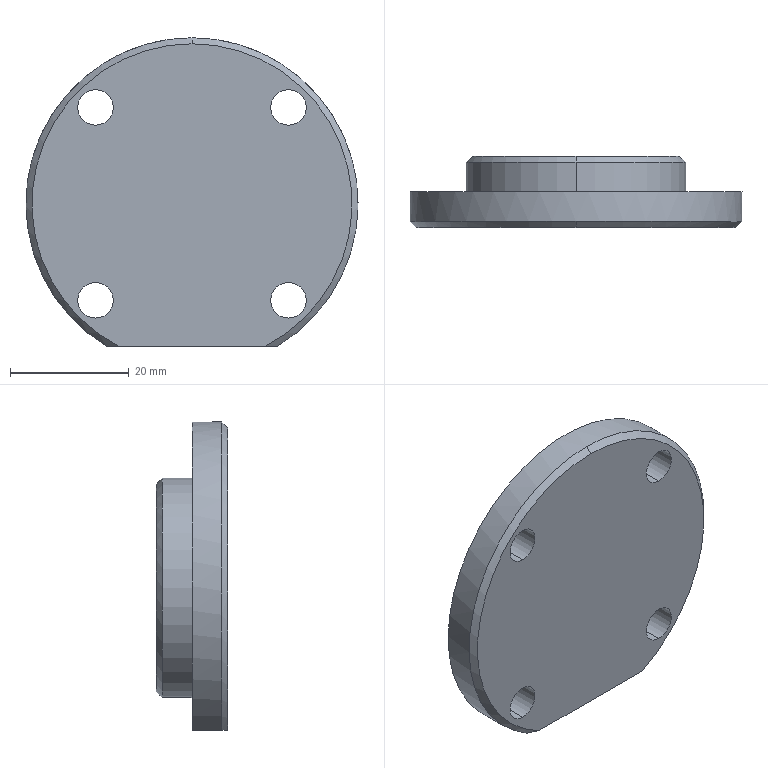Part | SolidWorks | features ICE 4, Chamfer 1, Extrusion 1, Fillet 1 | 1 solid | 24 faces | box 56 x 12 x 52 mm | volume 16065 mm3 | cylinder 13 | plane 5 | cone 4 | torus 2 | commonest cylinder face diameters 6 x8 29 x2 37 x2 56 x1
STEP:
#1=CARTESIAN_POINT('',(-16.263,0.,13.263));
#2=VERTEX_POINT('',#1);
#3=CARTESIAN_POINT('',(-16.263,0.,19.263));
#4=VERTEX_POINT('',#3);
#5=CARTESIAN_POINT('',(-16.263,0.,16.263));
#6=DIRECTION('',(0.,1.,0.));
#7=DIRECTION('',(0.,0.,1.));
#8=AXIS2_PLACEMENT_3D('',#5,#6,#7);
#9=CIRCLE('',#8,3.);
#10=EDGE_CURVE('',#2,#4,#9,.T.);
#11=ORIENTED_EDGE('',*,*,#10,.F.);
#12=CARTESIAN_POINT('',(-16.263,6.,13.263));
#13=VERTEX_POINT('',#12);
#14=CARTESIAN_POINT('',(-16.263,0.,13.263));
#15=DIRECTION('',(0.,1.,0.));
#16=VECTOR('',#15,1000.);
#17=LINE('',#14,#16);
#18=EDGE_CURVE('',#2,#13,#17,.T.);
#19=ORIENTED_EDGE('',*,*,#18,.T.);
#20=CARTESIAN_POINT('',(-16.263,6.,19.263));
#21=VERTEX_POINT('',#20);
#22=CARTESIAN_POINT('',(-16.263,6.,16.263));
#23=DIRECTION('',(0.,1.,0.));
#24=DIRECTION('',(0.,0.,1.));
#25=AXIS2_PLACEMENT_3D('',#22,#23,#24);
#26=CIRCLE('',#25,3.);
#27=EDGE_CURVE('',#13,#21,#26,.T.);
#28=ORIENTED_EDGE('',*,*,#27,.T.);
#29=CARTESIAN_POINT('',(-16.263,0.,19.263));
#30=DIRECTION('',(0.,1.,0.));
#31=VECTOR('',#30,1000.);
#32=LINE('',#29,#31);
#33=EDGE_CURVE('',#4,#21,#32,.T.);
#34=ORIENTED_EDGE('',*,*,#33,.F.);
#35=EDGE_LOOP('',(#11,#19,#28,#34));
#36=FACE_OUTER_BOUND('',#35,.T.);
#37=CARTESIAN_POINT('',(-16.263,0.,16.263));
#38=DIRECTION('',(0.,1.,0.));
#39=DIRECTION('',(0.,0.,1.));
#40=AXIS2_PLACEMENT_3D('',#37,#38,#39);
#41=CYLINDRICAL_SURFACE('',#40,3.);
#42=ADVANCED_FACE('',(#36),#41,.F.);
#43=CARTESIAN_POINT('',(16.263,0.,13.263));
#44=VERTEX_POINT('',#43);
#45=CARTESIAN_POINT('',(16.263,0.,19.263));
#46=VERTEX_POINT('',#45);
#47=CARTESIAN_POINT('',(16.263,0.,16.263));
#48=DIRECTION('',(0.,1.,0.));
#49=DIRECTION('',(0.,0.,1.));
#50=AXIS2_PLACEMENT_3D('',#47,#48,#49);
#51=CIRCLE('',#50,3.);
#52=EDGE_CURVE('',#44,#46,#51,.T.);
#53=ORIENTED_EDGE('',*,*,#52,.F.);
#54=CARTESIAN_POINT('',(16.263,6.,13.263));
#55=VERTEX_POINT('',#54);
#56=CARTESIAN_POINT('',(16.263,0.,13.263));
#57=DIRECTION('',(0.,1.,0.));
#58=VECTOR('',#57,1000.);
#59=LINE('',#56,#58);
#60=EDGE_CURVE('',#44,#55,#59,.T.);
#61=ORIENTED_EDGE('',*,*,#60,.T.);
#62=CARTESIAN_POINT('',(16.263,6.,19.263));
#63=VERTEX_POINT('',#62);
#64=CARTESIAN_POINT('',(16.263,6.,16.263));
#65=DIRECTION('',(0.,1.,0.));
#66=DIRECTION('',(0.,0.,1.));
#67=AXIS2_PLACEMENT_3D('',#64,#65,#66);
#68=CIRCLE('',#67,3.);
#69=EDGE_CURVE('',#55,#63,#68,.T.);
#70=ORIENTED_EDGE('',*,*,#69,.T.);
#71=CARTESIAN_POINT('',(16.263,0.,19.263));
#72=DIRECTION('',(0.,1.,0.));
#73=VECTOR('',#72,1000.);
#74=LINE('',#71,#73);
#75=EDGE_CURVE('',#46,#63,#74,.T.);
#76=ORIENTED_EDGE('',*,*,#75,.F.);
#77=EDGE_LOOP('',(#53,#61,#70,#76));
#78=FACE_OUTER_BOUND('',#77,.T.);
#79=CARTESIAN_POINT('',(16.263,0.,16.263));
#80=DIRECTION('',(0.,1.,0.));
#81=DIRECTION('',(0.,0.,1.));
#82=AXIS2_PLACEMENT_3D('',#79,#80,#81);
#83=CYLINDRICAL_SURFACE('',#82,3.);
#84=ADVANCED_FACE('',(#78),#83,.F.);
#85=CARTESIAN_POINT('',(16.263,0.,-19.263));
#86=VERTEX_POINT('',#85);
#87=CARTESIAN_POINT('',(16.263,0.,-13.263));
#88=VERTEX_POINT('',#87);
#89=CARTESIAN_POINT('',(16.263,0.,-16.263));
#90=DIRECTION('',(0.,1.,0.));
#91=DIRECTION('',(0.,0.,1.));
#92=AXIS2_PLACEMENT_3D('',#89,#90,#91);
#93=CIRCLE('',#92,3.);
#94=EDGE_CURVE('',#86,#88,#93,.T.);
#95=ORIENTED_EDGE('',*,*,#94,.F.);
#96=CARTESIAN_POINT('',(16.263,6.,-19.263));
#97=VERTEX_POINT('',#96);
#98=CARTESIAN_POINT('',(16.263,0.,-19.263));
#99=DIRECTION('',(0.,1.,0.));
#100=VECTOR('',#99,1000.);
#101=LINE('',#98,#100);
#102=EDGE_CURVE('',#86,#97,#101,.T.);
#103=ORIENTED_EDGE('',*,*,#102,.T.);
#104=CARTESIAN_POINT('',(16.263,6.,-13.263));
#105=VERTEX_POINT('',#104);
#106=CARTESIAN_POINT('',(16.263,6.,-16.263));
#107=DIRECTION('',(0.,1.,0.));
#108=DIRECTION('',(0.,0.,1.));
#109=AXIS2_PLACEMENT_3D('',#106,#107,#108);
#110=CIRCLE('',#109,3.);
#111=EDGE_CURVE('',#97,#105,#110,.T.);
#112=ORIENTED_EDGE('',*,*,#111,.T.);
#113=CARTESIAN_POINT('',(16.263,0.,-13.263));
#114=DIRECTION('',(0.,1.,0.));
#115=VECTOR('',#114,1000.);
#116=LINE('',#113,#115);
#117=EDGE_CURVE('',#88,#105,#116,.T.);
#118=ORIENTED_EDGE('',*,*,#117,.F.);
#119=EDGE_LOOP('',(#95,#103,#112,#118));
#120=FACE_OUTER_BOUND('',#119,.T.);
#121=CARTESIAN_POINT('',(16.263,0.,-16.263));
#122=DIRECTION('',(0.,1.,0.));
#123=DIRECTION('',(0.,0.,1.));
#124=AXIS2_PLACEMENT_3D('',#121,#122,#123);
#125=CYLINDRICAL_SURFACE('',#124,3.);
#126=ADVANCED_FACE('',(#120),#125,.F.);
#127=CARTESIAN_POINT('',(-16.263,0.,-19.263));
#128=VERTEX_POINT('',#127);
#129=CARTESIAN_POINT('',(-16.263,0.,-13.263));
#130=VERTEX_POINT('',#129);
#131=CARTESIAN_POINT('',(-16.263,0.,-16.263));
#132=DIRECTION('',(0.,1.,0.));
#133=DIRECTION('',(0.,0.,1.));
#134=AXIS2_PLACEMENT_3D('',#131,#132,#133);
#135=CIRCLE('',#134,3.);
#136=EDGE_CURVE('',#128,#130,#135,.T.);
#137=ORIENTED_EDGE('',*,*,#136,.F.);
#138=CARTESIAN_POINT('',(-16.263,6.,-19.263));
#139=VERTEX_POINT('',#138);
#140=CARTESIAN_POINT('',(-16.263,0.,-19.263));
#141=DIRECTION('',(0.,1.,0.));
#142=VECTOR('',#141,1000.);
#143=LINE('',#140,#142);
#144=EDGE_CURVE('',#128,#139,#143,.T.);
#145=ORIENTED_EDGE('',*,*,#144,.T.);
#146=CARTESIAN_POINT('',(-16.263,6.,-13.263));
#147=VERTEX_POINT('',#146);
#148=CARTESIAN_POINT('',(-16.263,6.,-16.263));
#149=DIRECTION('',(0.,1.,0.));
#150=DIRECTION('',(0.,0.,1.));
#151=AXIS2_PLACEMENT_3D('',#148,#149,#150);
#152=CIRCLE('',#151,3.);
#153=EDGE_CURVE('',#139,#147,#152,.T.);
#154=ORIENTED_EDGE('',*,*,#153,.T.);
#155=CARTESIAN_POINT('',(-16.263,0.,-13.263));
#156=DIRECTION('',(0.,1.,0.));
#157=VECTOR('',#156,1000.);
#158=LINE('',#155,#157);
#159=EDGE_CURVE('',#130,#147,#158,.T.);
#160=ORIENTED_EDGE('',*,*,#159,.F.);
#161=EDGE_LOOP('',(#137,#145,#154,#160));
#162=FACE_OUTER_BOUND('',#161,.T.);
#163=CARTESIAN_POINT('',(-16.263,0.,-16.263));
#164=DIRECTION('',(0.,1.,0.));
#165=DIRECTION('',(0.,0.,1.));
#166=AXIS2_PLACEMENT_3D('',#163,#164,#165);
#167=CYLINDRICAL_SURFACE('',#166,3.);
#168=ADVANCED_FACE('',(#162),#167,.F.);
#169=CARTESIAN_POINT('',(0.,12.,17.5));
#170=VERTEX_POINT('',#169);
#171=CARTESIAN_POINT('',(0.,12.,-17.5));
#172=VERTEX_POINT('',#171);
#173=CARTESIAN_POINT('',(0.,12.,0.));
#174=DIRECTION('',(0.,1.,0.));
#175=DIRECTION('',(0.,0.,1.));
#176=AXIS2_PLACEMENT_3D('',#173,#174,#175);
#177=CIRCLE('',#176,17.5);
#178=EDGE_CURVE('',#170,#172,#177,.T.);
#179=ORIENTED_EDGE('',*,*,#178,.F.);
#180=CARTESIAN_POINT('',(0.,11.,18.5));
#181=VERTEX_POINT('',#180);
#182=CARTESIAN_POINT('',(0.,12.,17.5));
#183=DIRECTION('',(0.,-0.7071,0.7071));
#184=VECTOR('',#183,1000.);
#185=LINE('',#182,#184);
#186=EDGE_CURVE('',#170,#181,#185,.T.);
#187=ORIENTED_EDGE('',*,*,#186,.T.);
#188=CARTESIAN_POINT('',(0.,11.,-18.5));
#189=VERTEX_POINT('',#188);
#190=CARTESIAN_POINT('',(0.,11.,0.));
#191=DIRECTION('',(0.,-1.,0.));
#192=DIRECTION('',(0.,0.,1.));
#193=AXIS2_PLACEMENT_3D('',#190,#191,#192);
#194=CIRCLE('',#193,18.5);
#195=EDGE_CURVE('',#189,#181,#194,.T.);
#196=ORIENTED_EDGE('',*,*,#195,.F.);
#197=CARTESIAN_POINT('',(0.,12.,-17.5));
#198=DIRECTION('',(0.,-0.7071,-0.7071));
#199=VECTOR('',#198,1000.);
#200=LINE('',#197,#199);
#201=EDGE_CURVE('',#172,#189,#200,.T.);
#202=ORIENTED_EDGE('',*,*,#201,.F.);
#203=EDGE_LOOP('',(#179,#187,#196,#202));
#204=FACE_OUTER_BOUND('',#203,.T.);
#205=CARTESIAN_POINT('',(0.,12.,0.));
#206=DIRECTION('',(0.,-1.,0.));
#207=DIRECTION('',(0.,0.,-1.));
#208=AXIS2_PLACEMENT_3D('',#205,#206,#207);
#209=CONICAL_SURFACE('',#208,17.5,0.7854);
#210=ADVANCED_FACE('',(#204),#209,.T.);
#211=CARTESIAN_POINT('',(0.,0.,27.));
#212=VERTEX_POINT('',#211);
#213=CARTESIAN_POINT('',(-12.369,0.,-24.));
#214=VERTEX_POINT('',#213);
#215=CARTESIAN_POINT('',(0.,0.,0.));
#216=DIRECTION('',(0.,-1.,0.));
#217=DIRECTION('',(0.,0.,1.));
#218=AXIS2_PLACEMENT_3D('',#215,#216,#217);
#219=CIRCLE('',#218,27.);
#220=EDGE_CURVE('',#212,#214,#219,.T.);
#221=ORIENTED_EDGE('',*,*,#220,.F.);
#222=CARTESIAN_POINT('',(0.,1.,28.));
#223=VERTEX_POINT('',#222);
#224=CARTESIAN_POINT('',(0.,1.,28.));
#225=DIRECTION('',(0.,0.7071,0.7071));
#226=VECTOR('',#225,1000.);
#227=LINE('',#224,#226);
#228=EDGE_CURVE('',#212,#223,#227,.T.);
#229=ORIENTED_EDGE('',*,*,#228,.T.);
#230=CARTESIAN_POINT('',(-14.422,1.,-24.));
#231=VERTEX_POINT('',#230);
#232=CARTESIAN_POINT('',(0.,1.,0.));
#233=DIRECTION('',(0.,1.,0.));
#234=DIRECTION('',(0.,0.,1.));
#235=AXIS2_PLACEMENT_3D('',#232,#233,#234);
#236=CIRCLE('',#235,28.);
#237=EDGE_CURVE('',#231,#223,#236,.T.);
#238=ORIENTED_EDGE('',*,*,#237,.F.);
#239=CARTESIAN_POINT('',(-12.369,0.,-24.));
#240=CARTESIAN_POINT('',(-13.06,0.3166,-24.));
#241=CARTESIAN_POINT('',(-13.744,0.6508,-24.));
#242=CARTESIAN_POINT('',(-14.422,1.,-24.));
#243=B_SPLINE_CURVE_WITH_KNOTS('',3,(#239,#240,#241,#242),.UNSPECIFIED.,.F.,.F.,(4,4),(0.02762,0.02986),.UNSPECIFIED.);
#244=EDGE_CURVE('',#214,#231,#243,.T.);
#245=ORIENTED_EDGE('',*,*,#244,.F.);
#246=EDGE_LOOP('',(#221,#229,#238,#245));
#247=FACE_OUTER_BOUND('',#246,.T.);
#248=CARTESIAN_POINT('',(0.,1.,0.));
#249=DIRECTION('',(0.,1.,0.));
#250=DIRECTION('',(0.,0.,1.));
#251=AXIS2_PLACEMENT_3D('',#248,#249,#250);
#252=CONICAL_SURFACE('',#251,28.,0.7854);
#253=ADVANCED_FACE('',(#247),#252,.T.);
#254=CARTESIAN_POINT('',(0.,6.,-12.5));
#255=VERTEX_POINT('',#254);
#256=CARTESIAN_POINT('',(0.,6.,12.5));
#257=VERTEX_POINT('',#256);
#258=CARTESIAN_POINT('',(0.,6.,0.));
#259=DIRECTION('',(0.,1.,0.));
#260=DIRECTION('',(0.,0.,1.));
#261=AXIS2_PLACEMENT_3D('',#258,#259,#260);
#262=CIRCLE('',#261,12.5);
#263=EDGE_CURVE('',#255,#257,#262,.T.);
#264=ORIENTED_EDGE('',*,*,#263,.F.);
#265=CARTESIAN_POINT('',(0.,8.,-14.5));
#266=VERTEX_POINT('',#265);
#267=CARTESIAN_POINT('',(0.,8.,-12.5));
#268=DIRECTION('',(1.,0.,0.));
#269=DIRECTION('',(0.,0.,-1.));
#270=AXIS2_PLACEMENT_3D('',#267,#268,#269);
#271=CIRCLE('',#270,2.);
#272=EDGE_CURVE('',#255,#266,#271,.T.);
#273=ORIENTED_EDGE('',*,*,#272,.T.);
#274=CARTESIAN_POINT('',(0.,8.,14.5));
#275=VERTEX_POINT('',#274);
#276=CARTESIAN_POINT('',(0.,8.,0.));
#277=DIRECTION('',(0.,-1.,0.));
#278=DIRECTION('',(0.,0.,1.));
#279=AXIS2_PLACEMENT_3D('',#276,#277,#278);
#280=CIRCLE('',#279,14.5);
#281=EDGE_CURVE('',#275,#266,#280,.T.);
#282=ORIENTED_EDGE('',*,*,#281,.F.);
#283=CARTESIAN_POINT('',(0.,8.,12.5));
#284=DIRECTION('',(-1.,0.,0.));
#285=DIRECTION('',(0.,0.,1.));
#286=AXIS2_PLACEMENT_3D('',#283,#284,#285);
#287=CIRCLE('',#286,2.);
#288=EDGE_CURVE('',#257,#275,#287,.T.);
#289=ORIENTED_EDGE('',*,*,#288,.F.);
#290=EDGE_LOOP('',(#264,#273,#282,#289));
#291=FACE_OUTER_BOUND('',#290,.T.);
#292=CARTESIAN_POINT('',(0.,8.,0.));
#293=DIRECTION('',(0.,1.,0.));
#294=DIRECTION('',(0.,0.,1.));
#295=AXIS2_PLACEMENT_3D('',#292,#293,#294);
#296=TOROIDAL_SURFACE('',#295,12.5,2.);
#297=ADVANCED_FACE('',(#291),#296,.F.);
#298=ORIENTED_EDGE('',*,*,#281,.T.);
#299=CARTESIAN_POINT('',(0.,12.,-14.5));
#300=VERTEX_POINT('',#299);
#301=CARTESIAN_POINT('',(0.,6.,-14.5));
#302=DIRECTION('',(0.,1.,0.));
#303=VECTOR('',#302,1000.);
#304=LINE('',#301,#303);
#305=EDGE_CURVE('',#266,#300,#304,.T.);
#306=ORIENTED_EDGE('',*,*,#305,.T.);
#307=CARTESIAN_POINT('',(0.,12.,14.5));
#308=VERTEX_POINT('',#307);
#309=CARTESIAN_POINT('',(0.,12.,0.));
#310=DIRECTION('',(0.,1.,0.));
#311=DIRECTION('',(0.,0.,1.));
#312=AXIS2_PLACEMENT_3D('',#309,#310,#311);
#313=CIRCLE('',#312,14.5);
#314=EDGE_CURVE('',#300,#308,#313,.T.);
#315=ORIENTED_EDGE('',*,*,#314,.T.);
#316=CARTESIAN_POINT('',(0.,6.,14.5));
#317=DIRECTION('',(0.,1.,0.));
#318=VECTOR('',#317,1000.);
#319=LINE('',#316,#318);
#320=EDGE_CURVE('',#275,#308,#319,.T.);
#321=ORIENTED_EDGE('',*,*,#320,.F.);
#322=EDGE_LOOP('',(#298,#306,#315,#321));
#323=FACE_OUTER_BOUND('',#322,.T.);
#324=CARTESIAN_POINT('',(0.,6.,0.));
#325=DIRECTION('',(0.,1.,0.));
#326=DIRECTION('',(0.,0.,1.));
#327=AXIS2_PLACEMENT_3D('',#324,#325,#326);
#328=CYLINDRICAL_SURFACE('',#327,14.5);
#329=ADVANCED_FACE('',(#323),#328,.F.);
#330=ORIENTED_EDGE('',*,*,#195,.T.);
#331=CARTESIAN_POINT('',(0.,6.,18.5));
#332=VERTEX_POINT('',#331);
#333=CARTESIAN_POINT('',(0.,12.,18.5));
#334=DIRECTION('',(0.,-1.,0.));
#335=VECTOR('',#334,1000.);
#336=LINE('',#333,#335);
#337=EDGE_CURVE('',#181,#332,#336,.T.);
#338=ORIENTED_EDGE('',*,*,#337,.T.);
#339=CARTESIAN_POINT('',(0.,6.,-18.5));
#340=VERTEX_POINT('',#339);
#341=CARTESIAN_POINT('',(0.,6.,0.));
#342=DIRECTION('',(0.,1.,0.));
#343=DIRECTION('',(0.,0.,1.));
#344=AXIS2_PLACEMENT_3D('',#341,#342,#343);
#345=CIRCLE('',#344,18.5);
#346=EDGE_CURVE('',#332,#340,#345,.T.);
#347=ORIENTED_EDGE('',*,*,#346,.T.);
#348=CARTESIAN_POINT('',(0.,12.,-18.5));
#349=DIRECTION('',(0.,-1.,0.));
#350=VECTOR('',#349,1000.);
#351=LINE('',#348,#350);
#352=EDGE_CURVE('',#189,#340,#351,.T.);
#353=ORIENTED_EDGE('',*,*,#352,.F.);
#354=EDGE_LOOP('',(#330,#338,#347,#353));
#355=FACE_OUTER_BOUND('',#354,.T.);
#356=CARTESIAN_POINT('',(0.,12.,0.));
#357=DIRECTION('',(0.,-1.,0.));
#358=DIRECTION('',(0.,0.,-1.));
#359=AXIS2_PLACEMENT_3D('',#356,#357,#358);
#360=CYLINDRICAL_SURFACE('',#359,18.5);
#361=ADVANCED_FACE('',(#355),#360,.T.);
#362=CARTESIAN_POINT('',(-14.422,6.,-24.));
#363=VERTEX_POINT('',#362);
#364=CARTESIAN_POINT('',(14.422,6.,-24.));
#365=VERTEX_POINT('',#364);
#366=CARTESIAN_POINT('',(0.,6.,0.));
#367=DIRECTION('',(0.,1.,0.));
#368=DIRECTION('',(0.,0.,1.));
#369=AXIS2_PLACEMENT_3D('',#366,#367,#368);
#370=CIRCLE('',#369,28.);
#371=EDGE_CURVE('',#363,#365,#370,.T.);
#372=ORIENTED_EDGE('',*,*,#371,.F.);
#373=CARTESIAN_POINT('',(-14.422,6.,-24.));
#374=DIRECTION('',(0.,-1.,0.));
#375=VECTOR('',#374,1000.);
#376=LINE('',#373,#375);
#377=EDGE_CURVE('',#363,#231,#376,.T.);
#378=ORIENTED_EDGE('',*,*,#377,.T.);
#379=ORIENTED_EDGE('',*,*,#237,.T.);
#380=CARTESIAN_POINT('',(14.422,1.,-24.));
#381=VERTEX_POINT('',#380);
#382=CARTESIAN_POINT('',(0.,1.,0.));
#383=DIRECTION('',(0.,1.,0.));
#384=DIRECTION('',(0.,0.,1.));
#385=AXIS2_PLACEMENT_3D('',#382,#383,#384);
#386=CIRCLE('',#385,28.);
#387=EDGE_CURVE('',#223,#381,#386,.T.);
#388=ORIENTED_EDGE('',*,*,#387,.T.);
#389=CARTESIAN_POINT('',(14.422,6.,-24.));
#390=DIRECTION('',(0.,1.,0.));
#391=VECTOR('',#390,1000.);
#392=LINE('',#389,#391);
#393=EDGE_CURVE('',#381,#365,#392,.T.);
#394=ORIENTED_EDGE('',*,*,#393,.T.);
#395=EDGE_LOOP('',(#372,#378,#379,#388,#394));
#396=FACE_OUTER_BOUND('',#395,.T.);
#397=CARTESIAN_POINT('',(0.,6.,0.));
#398=DIRECTION('',(0.,-1.,0.));
#399=DIRECTION('',(0.,0.,-1.));
#400=AXIS2_PLACEMENT_3D('',#397,#398,#399);
#401=CYLINDRICAL_SURFACE('',#400,28.);
#402=ADVANCED_FACE('',(#396),#401,.T.);
#403=CARTESIAN_POINT('',(-21.212,6.,-24.));
#404=DIRECTION('',(1.,0.,0.));
#405=VECTOR('',#404,1000.);
#406=LINE('',#403,#405);
#407=EDGE_CURVE('',#363,#365,#406,.T.);
#408=ORIENTED_EDGE('',*,*,#407,.F.);
#409=ORIENTED_EDGE('',*,*,#371,.T.);
#410=EDGE_LOOP('',(#408,#409));
#411=FACE_OUTER_BOUND('',#410,.T.);
#412=CARTESIAN_POINT('',(-16.263,6.,16.263));
#413=DIRECTION('',(0.,1.,0.));
#414=DIRECTION('',(0.,0.,1.));
#415=AXIS2_PLACEMENT_3D('',#412,#413,#414);
#416=CIRCLE('',#415,3.);
#417=EDGE_CURVE('',#21,#13,#416,.T.);
#418=ORIENTED_EDGE('',*,*,#417,.F.);
#419=ORIENTED_EDGE('',*,*,#27,.F.);
#420=EDGE_LOOP('',(#418,#419));
#421=FACE_BOUND('',#420,.T.);
#422=CARTESIAN_POINT('',(16.263,6.,16.263));
#423=DIRECTION('',(0.,1.,0.));
#424=DIRECTION('',(0.,0.,1.));
#425=AXIS2_PLACEMENT_3D('',#422,#423,#424);
#426=CIRCLE('',#425,3.);
#427=EDGE_CURVE('',#63,#55,#426,.T.);
#428=ORIENTED_EDGE('',*,*,#427,.F.);
#429=ORIENTED_EDGE('',*,*,#69,.F.);
#430=EDGE_LOOP('',(#428,#429));
#431=FACE_BOUND('',#430,.T.);
#432=CARTESIAN_POINT('',(16.263,6.,-16.263));
#433=DIRECTION('',(0.,1.,0.));
#434=DIRECTION('',(0.,0.,1.));
#435=AXIS2_PLACEMENT_3D('',#432,#433,#434);
#436=CIRCLE('',#435,3.);
#437=EDGE_CURVE('',#105,#97,#436,.T.);
#438=ORIENTED_EDGE('',*,*,#437,.F.);
#439=ORIENTED_EDGE('',*,*,#111,.F.);
#440=EDGE_LOOP('',(#438,#439));
#441=FACE_BOUND('',#440,.T.);
#442=CARTESIAN_POINT('',(-16.263,6.,-16.263));
#443=DIRECTION('',(0.,1.,0.));
#444=DIRECTION('',(0.,0.,1.));
#445=AXIS2_PLACEMENT_3D('',#442,#443,#444);
#446=CIRCLE('',#445,3.);
#447=EDGE_CURVE('',#147,#139,#446,.T.);
#448=ORIENTED_EDGE('',*,*,#447,.F.);
#449=ORIENTED_EDGE('',*,*,#153,.F.);
#450=EDGE_LOOP('',(#448,#449));
#451=FACE_BOUND('',#450,.T.);
#452=CARTESIAN_POINT('',(0.,6.,0.));
#453=DIRECTION('',(0.,1.,0.));
#454=DIRECTION('',(0.,0.,1.));
#455=AXIS2_PLACEMENT_3D('',#452,#453,#454);
#456=CIRCLE('',#455,18.5);
#457=EDGE_CURVE('',#340,#332,#456,.T.);
#458=ORIENTED_EDGE('',*,*,#457,.F.);
#459=ORIENTED_EDGE('',*,*,#346,.F.);
#460=EDGE_LOOP('',(#458,#459));
#461=FACE_BOUND('',#460,.T.);
#462=CARTESIAN_POINT('',(0.,6.,0.));
#463=DIRECTION('',(0.,1.,0.));
#464=DIRECTION('',(0.,0.,1.));
#465=AXIS2_PLACEMENT_3D('',#462,#463,#464);
#466=PLANE('',#465);
#467=ADVANCED_FACE('',(#411,#421,#431,#441,#451,#461),#466,.T.);
#468=CARTESIAN_POINT('',(-16.263,0.,16.263));
#469=DIRECTION('',(0.,1.,0.));
#470=DIRECTION('',(0.,0.,1.));
#471=AXIS2_PLACEMENT_3D('',#468,#469,#470);
#472=CIRCLE('',#471,3.);
#473=EDGE_CURVE('',#4,#2,#472,.T.);
#474=ORIENTED_EDGE('',*,*,#473,.T.);
#475=ORIENTED_EDGE('',*,*,#10,.T.);
#476=EDGE_LOOP('',(#474,#475));
#477=FACE_BOUND('',#476,.T.);
#478=CARTESIAN_POINT('',(16.263,0.,16.263));
#479=DIRECTION('',(0.,1.,0.));
#480=DIRECTION('',(0.,0.,1.));
#481=AXIS2_PLACEMENT_3D('',#478,#479,#480);
#482=CIRCLE('',#481,3.);
#483=EDGE_CURVE('',#46,#44,#482,.T.);
#484=ORIENTED_EDGE('',*,*,#483,.T.);
#485=ORIENTED_EDGE('',*,*,#52,.T.);
#486=EDGE_LOOP('',(#484,#485));
#487=FACE_BOUND('',#486,.T.);
#488=CARTESIAN_POINT('',(16.263,0.,-16.263));
#489=DIRECTION('',(0.,1.,0.));
#490=DIRECTION('',(0.,0.,1.));
#491=AXIS2_PLACEMENT_3D('',#488,#489,#490);
#492=CIRCLE('',#491,3.);
#493=EDGE_CURVE('',#88,#86,#492,.T.);
#494=ORIENTED_EDGE('',*,*,#493,.T.);
#495=ORIENTED_EDGE('',*,*,#94,.T.);
#496=EDGE_LOOP('',(#494,#495));
#497=FACE_BOUND('',#496,.T.);
#498=CARTESIAN_POINT('',(-16.263,0.,-16.263));
#499=DIRECTION('',(0.,1.,0.));
#500=DIRECTION('',(0.,0.,1.));
#501=AXIS2_PLACEMENT_3D('',#498,#499,#500);
#502=CIRCLE('',#501,3.);
#503=EDGE_CURVE('',#130,#128,#502,.T.);
#504=ORIENTED_EDGE('',*,*,#503,.T.);
#505=ORIENTED_EDGE('',*,*,#136,.T.);
#506=EDGE_LOOP('',(#504,#505));
#507=FACE_BOUND('',#506,.T.);
#508=CARTESIAN_POINT('',(12.369,0.,-24.));
#509=VERTEX_POINT('',#508);
#510=CARTESIAN_POINT('',(0.,0.,0.));
#511=DIRECTION('',(0.,-1.,0.));
#512=DIRECTION('',(0.,0.,1.));
#513=AXIS2_PLACEMENT_3D('',#510,#511,#512);
#514=CIRCLE('',#513,27.);
#515=EDGE_CURVE('',#509,#212,#514,.T.);
#516=ORIENTED_EDGE('',*,*,#515,.T.);
#517=ORIENTED_EDGE('',*,*,#220,.T.);
#518=CARTESIAN_POINT('',(-21.212,0.,-24.));
#519=DIRECTION('',(1.,0.,0.));
#520=VECTOR('',#519,1000.);
#521=LINE('',#518,#520);
#522=EDGE_CURVE('',#214,#509,#521,.T.);
#523=ORIENTED_EDGE('',*,*,#522,.T.);
#524=EDGE_LOOP('',(#516,#517,#523));
#525=FACE_OUTER_BOUND('',#524,.T.);
#526=CARTESIAN_POINT('',(0.,0.,0.));
#527=DIRECTION('',(0.,1.,0.));
#528=DIRECTION('',(0.,0.,1.));
#529=AXIS2_PLACEMENT_3D('',#526,#527,#528);
#530=PLANE('',#529);
#531=ADVANCED_FACE('',(#477,#487,#497,#507,#525),#530,.F.);
#532=ORIENTED_EDGE('',*,*,#337,.F.);
#533=CARTESIAN_POINT('',(0.,11.,0.));
#534=DIRECTION('',(0.,-1.,0.));
#535=DIRECTION('',(0.,0.,1.));
#536=AXIS2_PLACEMENT_3D('',#533,#534,#535);
#537=CIRCLE('',#536,18.5);
#538=EDGE_CURVE('',#181,#189,#537,.T.);
#539=ORIENTED_EDGE('',*,*,#538,.T.);
#540=ORIENTED_EDGE('',*,*,#352,.T.);
#541=ORIENTED_EDGE('',*,*,#457,.T.);
#542=EDGE_LOOP('',(#532,#539,#540,#541));
#543=FACE_OUTER_BOUND('',#542,.T.);
#544=CARTESIAN_POINT('',(0.,12.,0.));
#545=DIRECTION('',(0.,-1.,0.));
#546=DIRECTION('',(0.,0.,-1.));
#547=AXIS2_PLACEMENT_3D('',#544,#545,#546);
#548=CYLINDRICAL_SURFACE('',#547,18.5);
#549=ADVANCED_FACE('',(#543),#548,.T.);
#550=CARTESIAN_POINT('',(0.,12.,0.));
#551=DIRECTION('',(0.,1.,0.));
#552=DIRECTION('',(0.,0.,1.));
#553=AXIS2_PLACEMENT_3D('',#550,#551,#552);
#554=CIRCLE('',#553,17.5);
#555=EDGE_CURVE('',#172,#170,#554,.T.);
#556=ORIENTED_EDGE('',*,*,#555,.T.);
#557=ORIENTED_EDGE('',*,*,#178,.T.);
#558=EDGE_LOOP('',(#556,#557));
#559=FACE_OUTER_BOUND('',#558,.T.);
#560=CARTESIAN_POINT('',(0.,12.,0.));
#561=DIRECTION('',(0.,1.,0.));
#562=DIRECTION('',(0.,0.,1.));
#563=AXIS2_PLACEMENT_3D('',#560,#561,#562);
#564=CIRCLE('',#563,14.5);
#565=EDGE_CURVE('',#308,#300,#564,.T.);
#566=ORIENTED_EDGE('',*,*,#565,.F.);
#567=ORIENTED_EDGE('',*,*,#314,.F.);
#568=EDGE_LOOP('',(#566,#567));
#569=FACE_BOUND('',#568,.T.);
#570=CARTESIAN_POINT('',(0.,12.,0.));
#571=DIRECTION('',(0.,1.,0.));
#572=DIRECTION('',(0.,0.,1.));
#573=AXIS2_PLACEMENT_3D('',#570,#571,#572);
#574=PLANE('',#573);
#575=ADVANCED_FACE('',(#559,#569),#574,.T.);
#576=ORIENTED_EDGE('',*,*,#305,.F.);
#577=CARTESIAN_POINT('',(0.,8.,0.));
#578=DIRECTION('',(0.,-1.,0.));
#579=DIRECTION('',(0.,0.,1.));
#580=AXIS2_PLACEMENT_3D('',#577,#578,#579);
#581=CIRCLE('',#580,14.5);
#582=EDGE_CURVE('',#266,#275,#581,.T.);
#583=ORIENTED_EDGE('',*,*,#582,.T.);
#584=ORIENTED_EDGE('',*,*,#320,.T.);
#585=ORIENTED_EDGE('',*,*,#565,.T.);
#586=EDGE_LOOP('',(#576,#583,#584,#585));
#587=FACE_OUTER_BOUND('',#586,.T.);
#588=CARTESIAN_POINT('',(0.,6.,0.));
#589=DIRECTION('',(0.,1.,0.));
#590=DIRECTION('',(0.,0.,1.));
#591=AXIS2_PLACEMENT_3D('',#588,#589,#590);
#592=CYLINDRICAL_SURFACE('',#591,14.5);
#593=ADVANCED_FACE('',(#587),#592,.F.);
#594=CARTESIAN_POINT('',(0.,6.,0.));
#595=DIRECTION('',(0.,1.,0.));
#596=DIRECTION('',(0.,0.,1.));
#597=AXIS2_PLACEMENT_3D('',#594,#595,#596);
#598=CIRCLE('',#597,12.5);
#599=EDGE_CURVE('',#257,#255,#598,.T.);
#600=ORIENTED_EDGE('',*,*,#599,.T.);
#601=ORIENTED_EDGE('',*,*,#263,.T.);
#602=EDGE_LOOP('',(#600,#601));
#603=FACE_OUTER_BOUND('',#602,.T.);
#604=CARTESIAN_POINT('',(0.,6.,0.));
#605=DIRECTION('',(0.,1.,0.));
#606=DIRECTION('',(0.,0.,1.));
#607=AXIS2_PLACEMENT_3D('',#604,#605,#606);
#608=PLANE('',#607);
#609=ADVANCED_FACE('',(#603),#608,.T.);
#610=ORIENTED_EDGE('',*,*,#272,.F.);
#611=ORIENTED_EDGE('',*,*,#599,.F.);
#612=ORIENTED_EDGE('',*,*,#288,.T.);
#613=ORIENTED_EDGE('',*,*,#582,.F.);
#614=EDGE_LOOP('',(#610,#611,#612,#613));
#615=FACE_OUTER_BOUND('',#614,.T.);
#616=CARTESIAN_POINT('',(0.,8.,0.));
#617=DIRECTION('',(0.,1.,0.));
#618=DIRECTION('',(0.,0.,1.));
#619=AXIS2_PLACEMENT_3D('',#616,#617,#618);
#620=TOROIDAL_SURFACE('',#619,12.5,2.);
#621=ADVANCED_FACE('',(#615),#620,.F.);
#622=ORIENTED_EDGE('',*,*,#228,.F.);
#623=ORIENTED_EDGE('',*,*,#515,.F.);
#624=CARTESIAN_POINT('',(14.422,1.,-24.));
#625=CARTESIAN_POINT('',(13.743,0.6502,-24.));
#626=CARTESIAN_POINT('',(13.059,0.316,-24.));
#627=CARTESIAN_POINT('',(12.369,0.,-24.));
#628=B_SPLINE_CURVE_WITH_KNOTS('',3,(#624,#625,#626,#627),.UNSPECIFIED.,.F.,.F.,(4,4),(0.000001506,0.002259),.UNSPECIFIED.);
#629=EDGE_CURVE('',#381,#509,#628,.T.);
#630=ORIENTED_EDGE('',*,*,#629,.F.);
#631=ORIENTED_EDGE('',*,*,#387,.F.);
#632=EDGE_LOOP('',(#622,#623,#630,#631));
#633=FACE_OUTER_BOUND('',#632,.T.);
#634=CARTESIAN_POINT('',(0.,1.,0.));
#635=DIRECTION('',(0.,1.,0.));
#636=DIRECTION('',(0.,0.,1.));
#637=AXIS2_PLACEMENT_3D('',#634,#635,#636);
#638=CONICAL_SURFACE('',#637,28.,0.7854);
#639=ADVANCED_FACE('',(#633),#638,.T.);
#640=ORIENTED_EDGE('',*,*,#186,.F.);
#641=ORIENTED_EDGE('',*,*,#555,.F.);
#642=ORIENTED_EDGE('',*,*,#201,.T.);
#643=ORIENTED_EDGE('',*,*,#538,.F.);
#644=EDGE_LOOP('',(#640,#641,#642,#643));
#645=FACE_OUTER_BOUND('',#644,.T.);
#646=CARTESIAN_POINT('',(0.,12.,0.));
#647=DIRECTION('',(0.,-1.,0.));
#648=DIRECTION('',(0.,0.,-1.));
#649=AXIS2_PLACEMENT_3D('',#646,#647,#648);
#650=CONICAL_SURFACE('',#649,17.5,0.7854);
#651=ADVANCED_FACE('',(#645),#650,.T.);
#652=ORIENTED_EDGE('',*,*,#144,.F.);
#653=ORIENTED_EDGE('',*,*,#503,.F.);
#654=ORIENTED_EDGE('',*,*,#159,.T.);
#655=ORIENTED_EDGE('',*,*,#447,.T.);
#656=EDGE_LOOP('',(#652,#653,#654,#655));
#657=FACE_OUTER_BOUND('',#656,.T.);
#658=CARTESIAN_POINT('',(-16.263,0.,-16.263));
#659=DIRECTION('',(0.,1.,0.));
#660=DIRECTION('',(0.,0.,1.));
#661=AXIS2_PLACEMENT_3D('',#658,#659,#660);
#662=CYLINDRICAL_SURFACE('',#661,3.);
#663=ADVANCED_FACE('',(#657),#662,.F.);
#664=ORIENTED_EDGE('',*,*,#102,.F.);
#665=ORIENTED_EDGE('',*,*,#493,.F.);
#666=ORIENTED_EDGE('',*,*,#117,.T.);
#667=ORIENTED_EDGE('',*,*,#437,.T.);
#668=EDGE_LOOP('',(#664,#665,#666,#667));
#669=FACE_OUTER_BOUND('',#668,.T.);
#670=CARTESIAN_POINT('',(16.263,0.,-16.263));
#671=DIRECTION('',(0.,1.,0.));
#672=DIRECTION('',(0.,0.,1.));
#673=AXIS2_PLACEMENT_3D('',#670,#671,#672);
#674=CYLINDRICAL_SURFACE('',#673,3.);
#675=ADVANCED_FACE('',(#669),#674,.F.);
#676=ORIENTED_EDGE('',*,*,#60,.F.);
#677=ORIENTED_EDGE('',*,*,#483,.F.);
#678=ORIENTED_EDGE('',*,*,#75,.T.);
#679=ORIENTED_EDGE('',*,*,#427,.T.);
#680=EDGE_LOOP('',(#676,#677,#678,#679));
#681=FACE_OUTER_BOUND('',#680,.T.);
#682=CARTESIAN_POINT('',(16.263,0.,16.263));
#683=DIRECTION('',(0.,1.,0.));
#684=DIRECTION('',(0.,0.,1.));
#685=AXIS2_PLACEMENT_3D('',#682,#683,#684);
#686=CYLINDRICAL_SURFACE('',#685,3.);
#687=ADVANCED_FACE('',(#681),#686,.F.);
#688=ORIENTED_EDGE('',*,*,#18,.F.);
#689=ORIENTED_EDGE('',*,*,#473,.F.);
#690=ORIENTED_EDGE('',*,*,#33,.T.);
#691=ORIENTED_EDGE('',*,*,#417,.T.);
#692=EDGE_LOOP('',(#688,#689,#690,#691));
#693=FACE_OUTER_BOUND('',#692,.T.);
#694=CARTESIAN_POINT('',(-16.263,0.,16.263));
#695=DIRECTION('',(0.,1.,0.));
#696=DIRECTION('',(0.,0.,1.));
#697=AXIS2_PLACEMENT_3D('',#694,#695,#696);
#698=CYLINDRICAL_SURFACE('',#697,3.);
#699=ADVANCED_FACE('',(#693),#698,.F.);
#700=ORIENTED_EDGE('',*,*,#629,.T.);
#701=ORIENTED_EDGE('',*,*,#522,.F.);
#702=ORIENTED_EDGE('',*,*,#244,.T.);
#703=ORIENTED_EDGE('',*,*,#377,.F.);
#704=ORIENTED_EDGE('',*,*,#407,.T.);
#705=ORIENTED_EDGE('',*,*,#393,.F.);
#706=EDGE_LOOP('',(#700,#701,#702,#703,#704,#705));
#707=FACE_OUTER_BOUND('',#706,.T.);
#708=CARTESIAN_POINT('',(-21.212,0.,-24.));
#709=DIRECTION('',(0.,0.,1.));
#710=DIRECTION('',(1.,0.,0.));
#711=AXIS2_PLACEMENT_3D('',#708,#709,#710);
#712=PLANE('',#711);
#713=ADVANCED_FACE('',(#707),#712,.F.);
#714=CLOSED_SHELL('',(#42,#84,#126,#168,#210,#253,#297,#329,#361,#402,#467,#531,#549,#575,#593,#609,#621,#639,#651,#663,#675,#687,#699,#713));
#715=MANIFOLD_SOLID_BREP('',#714);
#716=CARTESIAN_POINT('',(0.,0.,0.));
#717=DIRECTION('',(0.,0.,1.));
#718=DIRECTION('',(1.,0.,0.));
#719=AXIS2_PLACEMENT_3D('',#716,#717,#718);
#720=(LENGTH_UNIT()NAMED_UNIT(*)SI_UNIT(.MILLI.,.METRE.));
#721=UNCERTAINTY_MEASURE_WITH_UNIT(LENGTH_MEASURE(0.00001),#720,'','');
#722=(NAMED_UNIT(*)PLANE_ANGLE_UNIT()SI_UNIT($,.RADIAN.));
#723=(NAMED_UNIT(*)SI_UNIT($,.STERADIAN.)SOLID_ANGLE_UNIT());
#724=(GEOMETRIC_REPRESENTATION_CONTEXT(3)GLOBAL_UNCERTAINTY_ASSIGNED_CONTEXT((#721))GLOBAL_UNIT_ASSIGNED_CONTEXT((#720,#722,#723))REPRESENTATION_CONTEXT('',''));
#725=ADVANCED_BREP_SHAPE_REPRESENTATION('',(#715,#719),#724);